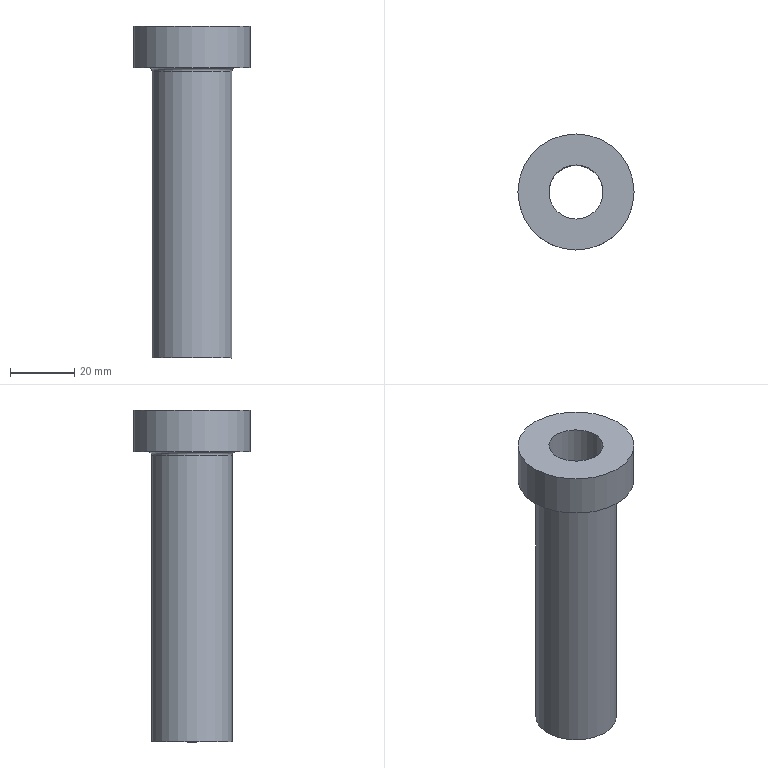Part | NX | features solid 2 | 1 solid | 7 faces | box 36 x 36 x 103 mm | volume 34596 mm3 | plane 3 | cylinder 3 | torus 1 | commonest cylinder face diameters 16.8 x1 25 x1 36 x1
STEP:
#1=CARTESIAN_POINT('',(-582.,651.501,240.));
#2=VERTEX_POINT('',#1);
#3=CARTESIAN_POINT('',(-582.,665.001,240.));
#4=DIRECTION('',(0.,0.,-1.));
#5=DIRECTION('',(0.,-1.,0.));
#6=AXIS2_PLACEMENT_3D('',#3,#4,#5);
#7=CIRCLE('',#6,13.5);
#8=EDGE_CURVE('',#2,#2,#7,.T.);
#9=ORIENTED_EDGE('',*,*,#8,.F.);
#10=EDGE_LOOP('',(#9));
#11=FACE_BOUND('',#10,.T.);
#12=CARTESIAN_POINT('',(-582.,683.001,240.));
#13=VERTEX_POINT('',#12);
#14=CARTESIAN_POINT('',(-582.,665.001,240.));
#15=DIRECTION('',(0.,0.,1.));
#16=DIRECTION('',(0.,1.,0.));
#17=AXIS2_PLACEMENT_3D('',#14,#15,#16);
#18=CIRCLE('',#17,18.);
#19=EDGE_CURVE('',#13,#13,#18,.T.);
#20=ORIENTED_EDGE('',*,*,#19,.F.);
#21=EDGE_LOOP('',(#20));
#22=FACE_BOUND('',#21,.T.);
#23=CARTESIAN_POINT('',(-582.,665.001,240.));
#24=DIRECTION('',(0.,0.,1.));
#25=DIRECTION('',(0.,-1.,0.));
#26=AXIS2_PLACEMENT_3D('',#23,#24,#25);
#27=PLANE('',#26);
#28=ADVANCED_FACE('',(#11,#22),#27,.F.);
#29=CARTESIAN_POINT('',(-582.,656.601,253.));
#30=VERTEX_POINT('',#29);
#31=CARTESIAN_POINT('',(-582.,665.001,253.));
#32=DIRECTION('',(0.,0.,-1.));
#33=DIRECTION('',(0.,-1.,0.));
#34=AXIS2_PLACEMENT_3D('',#31,#32,#33);
#35=CIRCLE('',#34,8.4);
#36=EDGE_CURVE('',#30,#30,#35,.T.);
#37=ORIENTED_EDGE('',*,*,#36,.T.);
#38=EDGE_LOOP('',(#37));
#39=FACE_BOUND('',#38,.T.);
#40=CARTESIAN_POINT('',(-582.,683.001,253.));
#41=VERTEX_POINT('',#40);
#42=CARTESIAN_POINT('',(-582.,665.001,253.));
#43=DIRECTION('',(0.,0.,1.));
#44=DIRECTION('',(0.,1.,0.));
#45=AXIS2_PLACEMENT_3D('',#42,#43,#44);
#46=CIRCLE('',#45,18.);
#47=EDGE_CURVE('',#41,#41,#46,.T.);
#48=ORIENTED_EDGE('',*,*,#47,.T.);
#49=EDGE_LOOP('',(#48));
#50=FACE_BOUND('',#49,.T.);
#51=CARTESIAN_POINT('',(-582.,665.001,253.));
#52=DIRECTION('',(0.,0.,1.));
#53=DIRECTION('',(0.,-1.,0.));
#54=AXIS2_PLACEMENT_3D('',#51,#52,#53);
#55=PLANE('',#54);
#56=ADVANCED_FACE('',(#39,#50),#55,.T.);
#57=ORIENTED_EDGE('',*,*,#19,.T.);
#58=EDGE_LOOP('',(#57));
#59=FACE_BOUND('',#58,.T.);
#60=ORIENTED_EDGE('',*,*,#47,.F.);
#61=EDGE_LOOP('',(#60));
#62=FACE_BOUND('',#61,.T.);
#63=CARTESIAN_POINT('',(-582.,665.001,253.));
#64=DIRECTION('',(0.,0.,-1.));
#65=DIRECTION('',(0.,1.,0.));
#66=AXIS2_PLACEMENT_3D('',#63,#64,#65);
#67=CYLINDRICAL_SURFACE('',#66,18.);
#68=ADVANCED_FACE('',(#59,#62),#67,.T.);
#69=CARTESIAN_POINT('',(-582.,673.401,150.));
#70=VERTEX_POINT('',#69);
#71=CARTESIAN_POINT('',(-582.,665.001,150.));
#72=DIRECTION('',(0.,0.,-1.));
#73=DIRECTION('',(0.,1.,0.));
#74=AXIS2_PLACEMENT_3D('',#71,#72,#73);
#75=CIRCLE('',#74,8.4);
#76=EDGE_CURVE('',#70,#70,#75,.T.);
#77=ORIENTED_EDGE('',*,*,#76,.F.);
#78=EDGE_LOOP('',(#77));
#79=FACE_BOUND('',#78,.T.);
#80=CARTESIAN_POINT('',(-582.,677.501,150.));
#81=VERTEX_POINT('',#80);
#82=CARTESIAN_POINT('',(-582.,665.001,150.));
#83=DIRECTION('',(0.,0.,-1.));
#84=DIRECTION('',(0.,1.,0.));
#85=AXIS2_PLACEMENT_3D('',#82,#83,#84);
#86=CIRCLE('',#85,12.5);
#87=EDGE_CURVE('',#81,#81,#86,.F.);
#88=ORIENTED_EDGE('',*,*,#87,.F.);
#89=EDGE_LOOP('',(#88));
#90=FACE_BOUND('',#89,.T.);
#91=CARTESIAN_POINT('',(-582.,665.001,150.));
#92=DIRECTION('',(0.,0.,-1.));
#93=DIRECTION('',(0.,1.,0.));
#94=AXIS2_PLACEMENT_3D('',#91,#92,#93);
#95=PLANE('',#94);
#96=ADVANCED_FACE('',(#79,#90),#95,.T.);
#97=CARTESIAN_POINT('',(-582.,652.501,239.));
#98=VERTEX_POINT('',#97);
#99=CARTESIAN_POINT('',(-582.,665.001,239.));
#100=DIRECTION('',(0.,0.,-1.));
#101=DIRECTION('',(0.,-1.,0.));
#102=AXIS2_PLACEMENT_3D('',#99,#100,#101);
#103=CIRCLE('',#102,12.5);
#104=EDGE_CURVE('',#98,#98,#103,.F.);
#105=ORIENTED_EDGE('',*,*,#104,.F.);
#106=EDGE_LOOP('',(#105));
#107=FACE_BOUND('',#106,.T.);
#108=ORIENTED_EDGE('',*,*,#87,.T.);
#109=EDGE_LOOP('',(#108));
#110=FACE_BOUND('',#109,.T.);
#111=CARTESIAN_POINT('',(-582.,665.001,240.));
#112=DIRECTION('',(0.,0.,-1.));
#113=DIRECTION('',(0.,1.,0.));
#114=AXIS2_PLACEMENT_3D('',#111,#112,#113);
#115=CYLINDRICAL_SURFACE('',#114,12.5);
#116=ADVANCED_FACE('',(#107,#110),#115,.T.);
#117=ORIENTED_EDGE('',*,*,#36,.F.);
#118=EDGE_LOOP('',(#117));
#119=FACE_BOUND('',#118,.T.);
#120=ORIENTED_EDGE('',*,*,#76,.T.);
#121=EDGE_LOOP('',(#120));
#122=FACE_BOUND('',#121,.T.);
#123=CARTESIAN_POINT('',(-582.,665.001,140.));
#124=DIRECTION('',(0.,0.,1.));
#125=DIRECTION('',(0.,-1.,0.));
#126=AXIS2_PLACEMENT_3D('',#123,#124,#125);
#127=CYLINDRICAL_SURFACE('',#126,8.4);
#128=ADVANCED_FACE('',(#119,#122),#127,.F.);
#129=ORIENTED_EDGE('',*,*,#8,.T.);
#130=EDGE_LOOP('',(#129));
#131=FACE_BOUND('',#130,.T.);
#132=ORIENTED_EDGE('',*,*,#104,.T.);
#133=EDGE_LOOP('',(#132));
#134=FACE_BOUND('',#133,.T.);
#135=CARTESIAN_POINT('',(-582.,665.001,239.));
#136=DIRECTION('',(0.,0.,1.));
#137=DIRECTION('',(0.,-1.,0.));
#138=AXIS2_PLACEMENT_3D('',#135,#136,#137);
#139=TOROIDAL_SURFACE('',#138,13.5,1.);
#140=ADVANCED_FACE('',(#131,#134),#139,.F.);
#141=CLOSED_SHELL('',(#28,#56,#68,#96,#116,#128,#140));
#142=MANIFOLD_SOLID_BREP('',#141);
#143=(LENGTH_UNIT()NAMED_UNIT(*)SI_UNIT(.MILLI.,.METRE.));
#144=UNCERTAINTY_MEASURE_WITH_UNIT(LENGTH_MEASURE(0.00001),#143,'','');
#145=(NAMED_UNIT(*)PLANE_ANGLE_UNIT()SI_UNIT($,.RADIAN.));
#146=(NAMED_UNIT(*)SI_UNIT($,.STERADIAN.)SOLID_ANGLE_UNIT());
#147=(GEOMETRIC_REPRESENTATION_CONTEXT(3)GLOBAL_UNCERTAINTY_ASSIGNED_CONTEXT((#144))GLOBAL_UNIT_ASSIGNED_CONTEXT((#143,#145,#146))REPRESENTATION_CONTEXT('',''));
#148=ADVANCED_BREP_SHAPE_REPRESENTATION('',(#142),#147);